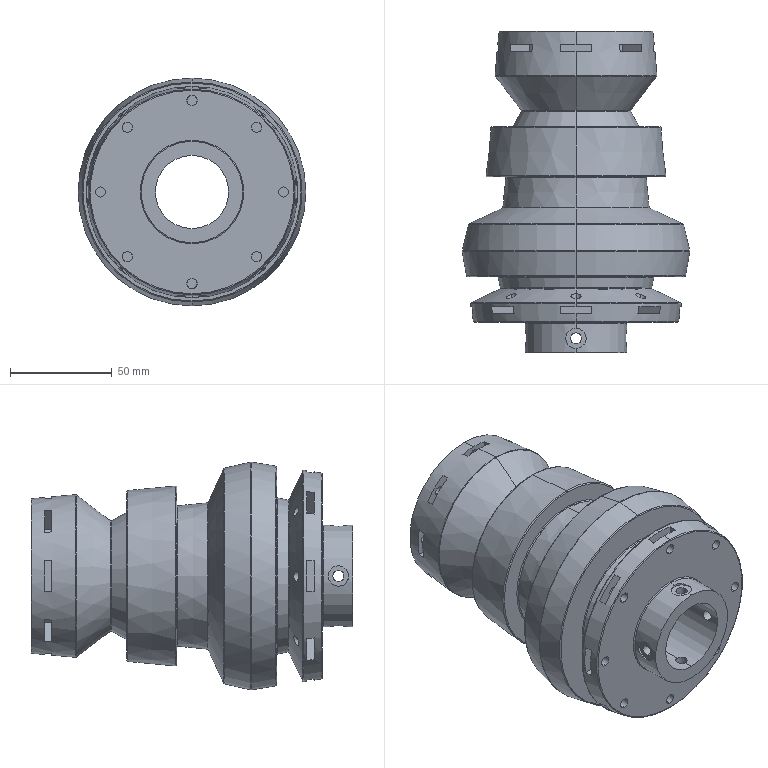Part | SolidWorks | features ICE 7, CirPattern 2, Fillet 1, Revolution 1 | 1 solid | 240 faces | box 111.982 x 158 x 111.982 mm | volume 684523 mm3 | plane 98 | cylinder 84 | torus 36 | cone 22 | commonest cylinder face diameters 5 x64 5.5 x8 10 x8 36 x2 50 x2